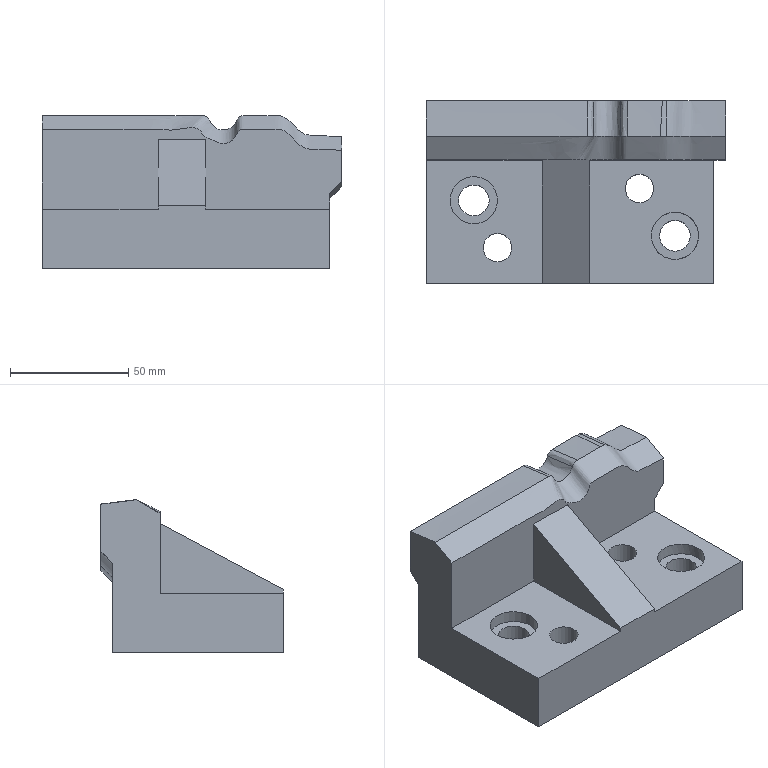Part | NX | features solid 2 | 1 solid | 33 faces | box 126.4 x 76.997 x 64.634 mm | volume 325487 mm3 | plane 14 | spline 13 | cylinder 6 | commonest cylinder face diameters 12 x2 13 x2 20 x2